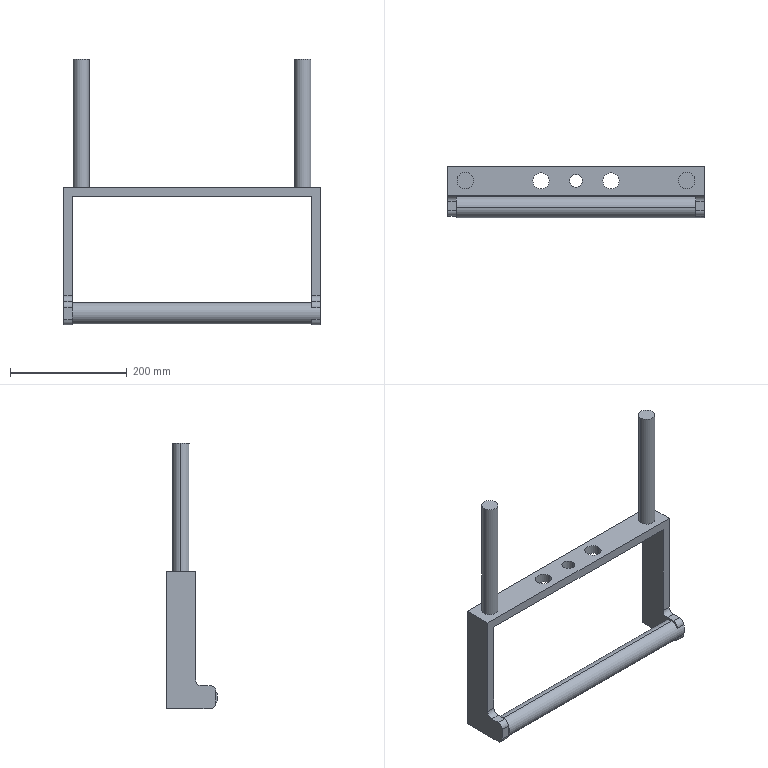Part | STEP file | 1 solid | 36 faces | box 440 x 88 x 456 mm | volume 1386399 mm3 | cylinder 18 | plane 18 | commonest cylinder face diameters 28 x8 20 x6 22.07 x2 36 x2